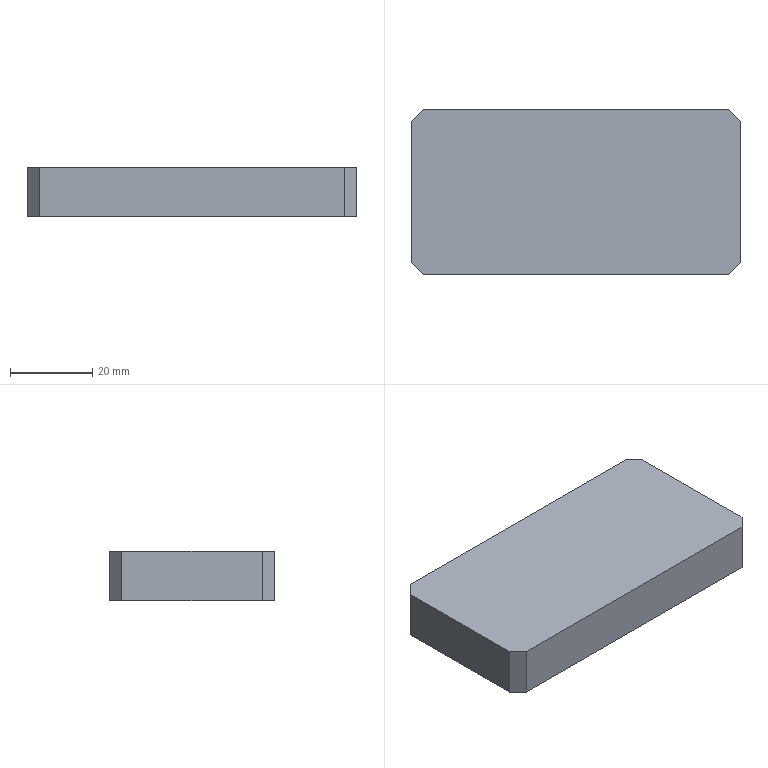Part | STEP file | 001-001-Small mounting plate | 1 solid | 10 faces | box 80 x 40 x 12 mm | volume 38184 mm3 | plane 10
STEP:
#1=CARTESIAN_POINT('',(0.,0.,0.));
#2=DIRECTION('',(0.,0.,1.));
#3=DIRECTION('',(1.,0.,0.));
#4=AXIS2_PLACEMENT_3D('',#1,#2,#3);
#5=CARTESIAN_POINT('',(-773.,430.,12.));
#6=VERTEX_POINT('',#5);
#7=CARTESIAN_POINT('',(-847.,430.,12.));
#8=VERTEX_POINT('',#7);
#9=CARTESIAN_POINT('',(-770.,430.,12.));
#10=DIRECTION('',(-1.,0.,0.));
#11=VECTOR('',#10,1.);
#12=LINE('',#9,#11);
#13=CARTESIAN_POINT('',(-770.,430.,12.));
#14=DIRECTION('',(0.,-1.,0.));
#15=DIRECTION('',(0.,0.,-1.));
#16=AXIS2_PLACEMENT_3D('',#13,#14,#15);
#17=PLANE('',#16);
#18=CARTESIAN_POINT('',(0.,0.));
#19=DIRECTION('',(0.,-1.));
#20=VECTOR('',#19,1.);
#21=LINE('',#18,#20);
#22=(GEOMETRIC_REPRESENTATION_CONTEXT(2)PARAMETRIC_REPRESENTATION_CONTEXT()REPRESENTATION_CONTEXT('',''));
#23=DEFINITIONAL_REPRESENTATION('',(#21),#22);
#24=PCURVE('',#17,#23);
#25=CARTESIAN_POINT('',(0.,0.,12.));
#26=DIRECTION('',(0.,0.,-1.));
#27=DIRECTION('',(-1.,0.,0.));
#28=AXIS2_PLACEMENT_3D('',#25,#26,#27);
#29=PLANE('',#28);
#30=CARTESIAN_POINT('',(770.,430.));
#31=DIRECTION('',(1.,0.));
#32=VECTOR('',#31,1.);
#33=LINE('',#30,#32);
#34=(GEOMETRIC_REPRESENTATION_CONTEXT(2)PARAMETRIC_REPRESENTATION_CONTEXT()REPRESENTATION_CONTEXT('',''));
#35=DEFINITIONAL_REPRESENTATION('',(#33),#34);
#36=PCURVE('',#29,#35);
#37=SURFACE_CURVE('',#12,(#24,#36),.PCURVE_S1.);
#38=EDGE_CURVE('',#6,#8,#37,.T.);
#39=ORIENTED_EDGE('',*,*,#38,.T.);
#40=CARTESIAN_POINT('',(-847.,430.,0.));
#41=VERTEX_POINT('',#40);
#42=CARTESIAN_POINT('',(-847.,430.,12.));
#43=DIRECTION('',(0.,0.,-1.));
#44=VECTOR('',#43,1.);
#45=LINE('',#42,#44);
#46=CARTESIAN_POINT('',(0.,-77.));
#47=DIRECTION('',(1.,0.));
#48=VECTOR('',#47,1.);
#49=LINE('',#46,#48);
#50=(GEOMETRIC_REPRESENTATION_CONTEXT(2)PARAMETRIC_REPRESENTATION_CONTEXT()REPRESENTATION_CONTEXT('',''));
#51=DEFINITIONAL_REPRESENTATION('',(#49),#50);
#52=PCURVE('',#17,#51);
#53=CARTESIAN_POINT('',(-847.,430.,12.));
#54=DIRECTION('',(0.7071,0.7071,0.));
#55=DIRECTION('',(0.,0.,-1.));
#56=AXIS2_PLACEMENT_3D('',#53,#54,#55);
#57=PLANE('',#56);
#58=CARTESIAN_POINT('',(0.,0.));
#59=DIRECTION('',(1.,0.));
#60=VECTOR('',#59,1.);
#61=LINE('',#58,#60);
#62=(GEOMETRIC_REPRESENTATION_CONTEXT(2)PARAMETRIC_REPRESENTATION_CONTEXT()REPRESENTATION_CONTEXT('',''));
#63=DEFINITIONAL_REPRESENTATION('',(#61),#62);
#64=PCURVE('',#57,#63);
#65=SURFACE_CURVE('',#45,(#52,#64),.PCURVE_S1.);
#66=EDGE_CURVE('',#8,#41,#65,.T.);
#67=ORIENTED_EDGE('',*,*,#66,.T.);
#68=CARTESIAN_POINT('',(-773.,430.,0.));
#69=VERTEX_POINT('',#68);
#70=CARTESIAN_POINT('',(-770.,430.,0.));
#71=DIRECTION('',(-1.,0.,0.));
#72=VECTOR('',#71,1.);
#73=LINE('',#70,#72);
#74=CARTESIAN_POINT('',(12.,0.));
#75=DIRECTION('',(0.,-1.));
#76=VECTOR('',#75,1.);
#77=LINE('',#74,#76);
#78=(GEOMETRIC_REPRESENTATION_CONTEXT(2)PARAMETRIC_REPRESENTATION_CONTEXT()REPRESENTATION_CONTEXT('',''));
#79=DEFINITIONAL_REPRESENTATION('',(#77),#78);
#80=PCURVE('',#17,#79);
#81=CARTESIAN_POINT('',(0.,0.,0.));
#82=DIRECTION('',(0.,0.,-1.));
#83=DIRECTION('',(-1.,0.,0.));
#84=AXIS2_PLACEMENT_3D('',#81,#82,#83);
#85=PLANE('',#84);
#86=CARTESIAN_POINT('',(770.,430.));
#87=DIRECTION('',(1.,0.));
#88=VECTOR('',#87,1.);
#89=LINE('',#86,#88);
#90=(GEOMETRIC_REPRESENTATION_CONTEXT(2)PARAMETRIC_REPRESENTATION_CONTEXT()REPRESENTATION_CONTEXT('',''));
#91=DEFINITIONAL_REPRESENTATION('',(#89),#90);
#92=PCURVE('',#85,#91);
#93=SURFACE_CURVE('',#73,(#80,#92),.PCURVE_S1.);
#94=EDGE_CURVE('',#69,#41,#93,.T.);
#95=ORIENTED_EDGE('',*,*,#94,.F.);
#96=CARTESIAN_POINT('',(-773.,430.,12.));
#97=DIRECTION('',(0.,0.,1.));
#98=VECTOR('',#97,1.);
#99=LINE('',#96,#98);
#100=CARTESIAN_POINT('',(0.,-3.));
#101=DIRECTION('',(-1.,0.));
#102=VECTOR('',#101,1.);
#103=LINE('',#100,#102);
#104=(GEOMETRIC_REPRESENTATION_CONTEXT(2)PARAMETRIC_REPRESENTATION_CONTEXT()REPRESENTATION_CONTEXT('',''));
#105=DEFINITIONAL_REPRESENTATION('',(#103),#104);
#106=PCURVE('',#17,#105);
#107=CARTESIAN_POINT('',(-770.,433.,12.));
#108=DIRECTION('',(0.7071,-0.7071,0.));
#109=DIRECTION('',(0.,0.,1.));
#110=AXIS2_PLACEMENT_3D('',#107,#108,#109);
#111=PLANE('',#110);
#112=CARTESIAN_POINT('',(0.,4.243));
#113=DIRECTION('',(1.,0.));
#114=VECTOR('',#113,1.);
#115=LINE('',#112,#114);
#116=(GEOMETRIC_REPRESENTATION_CONTEXT(2)PARAMETRIC_REPRESENTATION_CONTEXT()REPRESENTATION_CONTEXT('',''));
#117=DEFINITIONAL_REPRESENTATION('',(#115),#116);
#118=PCURVE('',#111,#117);
#119=SURFACE_CURVE('',#99,(#106,#118),.PCURVE_S1.);
#120=EDGE_CURVE('',#69,#6,#119,.T.);
#121=ORIENTED_EDGE('',*,*,#120,.T.);
#122=EDGE_LOOP('',(#39,#67,#95,#121));
#123=FACE_BOUND('',#122,.T.);
#124=ADVANCED_FACE('',(#123),#17,.T.);
#125=CARTESIAN_POINT('',(-770.,433.,12.));
#126=VERTEX_POINT('',#125);
#127=CARTESIAN_POINT('',(-770.,467.,12.));
#128=VERTEX_POINT('',#127);
#129=CARTESIAN_POINT('',(-770.,430.,12.));
#130=DIRECTION('',(0.,1.,0.));
#131=VECTOR('',#130,1.);
#132=LINE('',#129,#131);
#133=CARTESIAN_POINT('',(-770.,430.,12.));
#134=DIRECTION('',(-1.,0.,0.));
#135=DIRECTION('',(0.,0.,1.));
#136=AXIS2_PLACEMENT_3D('',#133,#134,#135);
#137=PLANE('',#136);
#138=CARTESIAN_POINT('',(0.,0.));
#139=DIRECTION('',(0.,1.));
#140=VECTOR('',#139,1.);
#141=LINE('',#138,#140);
#142=(GEOMETRIC_REPRESENTATION_CONTEXT(2)PARAMETRIC_REPRESENTATION_CONTEXT()REPRESENTATION_CONTEXT('',''));
#143=DEFINITIONAL_REPRESENTATION('',(#141),#142);
#144=PCURVE('',#137,#143);
#145=CARTESIAN_POINT('',(770.,430.));
#146=DIRECTION('',(0.,1.));
#147=VECTOR('',#146,1.);
#148=LINE('',#145,#147);
#149=(GEOMETRIC_REPRESENTATION_CONTEXT(2)PARAMETRIC_REPRESENTATION_CONTEXT()REPRESENTATION_CONTEXT('',''));
#150=DEFINITIONAL_REPRESENTATION('',(#148),#149);
#151=PCURVE('',#29,#150);
#152=SURFACE_CURVE('',#132,(#144,#151),.PCURVE_S1.);
#153=EDGE_CURVE('',#126,#128,#152,.T.);
#154=ORIENTED_EDGE('',*,*,#153,.F.);
#155=CARTESIAN_POINT('',(-770.,433.,0.));
#156=VERTEX_POINT('',#155);
#157=CARTESIAN_POINT('',(-770.,433.,0.));
#158=DIRECTION('',(0.,0.,-1.));
#159=VECTOR('',#158,1.);
#160=LINE('',#157,#159);
#161=CARTESIAN_POINT('',(-12.,3.));
#162=DIRECTION('',(-1.,0.));
#163=VECTOR('',#162,1.);
#164=LINE('',#161,#163);
#165=(GEOMETRIC_REPRESENTATION_CONTEXT(2)PARAMETRIC_REPRESENTATION_CONTEXT()REPRESENTATION_CONTEXT('',''));
#166=DEFINITIONAL_REPRESENTATION('',(#164),#165);
#167=PCURVE('',#137,#166);
#168=CARTESIAN_POINT('',(-12.,0.));
#169=DIRECTION('',(-1.,0.));
#170=VECTOR('',#169,1.);
#171=LINE('',#168,#170);
#172=(GEOMETRIC_REPRESENTATION_CONTEXT(2)PARAMETRIC_REPRESENTATION_CONTEXT()REPRESENTATION_CONTEXT('',''));
#173=DEFINITIONAL_REPRESENTATION('',(#171),#172);
#174=PCURVE('',#111,#173);
#175=SURFACE_CURVE('',#160,(#167,#174),.PCURVE_S1.);
#176=EDGE_CURVE('',#126,#156,#175,.T.);
#177=ORIENTED_EDGE('',*,*,#176,.T.);
#178=CARTESIAN_POINT('',(-770.,467.,0.));
#179=VERTEX_POINT('',#178);
#180=CARTESIAN_POINT('',(-770.,430.,0.));
#181=DIRECTION('',(0.,1.,0.));
#182=VECTOR('',#181,1.);
#183=LINE('',#180,#182);
#184=CARTESIAN_POINT('',(-12.,0.));
#185=DIRECTION('',(0.,1.));
#186=VECTOR('',#185,1.);
#187=LINE('',#184,#186);
#188=(GEOMETRIC_REPRESENTATION_CONTEXT(2)PARAMETRIC_REPRESENTATION_CONTEXT()REPRESENTATION_CONTEXT('',''));
#189=DEFINITIONAL_REPRESENTATION('',(#187),#188);
#190=PCURVE('',#137,#189);
#191=CARTESIAN_POINT('',(770.,430.));
#192=DIRECTION('',(0.,1.));
#193=VECTOR('',#192,1.);
#194=LINE('',#191,#193);
#195=(GEOMETRIC_REPRESENTATION_CONTEXT(2)PARAMETRIC_REPRESENTATION_CONTEXT()REPRESENTATION_CONTEXT('',''));
#196=DEFINITIONAL_REPRESENTATION('',(#194),#195);
#197=PCURVE('',#85,#196);
#198=SURFACE_CURVE('',#183,(#190,#197),.PCURVE_S1.);
#199=EDGE_CURVE('',#156,#179,#198,.T.);
#200=ORIENTED_EDGE('',*,*,#199,.T.);
#201=CARTESIAN_POINT('',(-770.,467.,12.));
#202=DIRECTION('',(0.,0.,1.));
#203=VECTOR('',#202,1.);
#204=LINE('',#201,#203);
#205=CARTESIAN_POINT('',(0.,37.));
#206=DIRECTION('',(1.,0.));
#207=VECTOR('',#206,1.);
#208=LINE('',#205,#207);
#209=(GEOMETRIC_REPRESENTATION_CONTEXT(2)PARAMETRIC_REPRESENTATION_CONTEXT()REPRESENTATION_CONTEXT('',''));
#210=DEFINITIONAL_REPRESENTATION('',(#208),#209);
#211=PCURVE('',#137,#210);
#212=CARTESIAN_POINT('',(-773.,470.,12.));
#213=DIRECTION('',(-0.7071,-0.7071,0.));
#214=DIRECTION('',(0.,0.,-1.));
#215=AXIS2_PLACEMENT_3D('',#212,#213,#214);
#216=PLANE('',#215);
#217=CARTESIAN_POINT('',(0.,4.243));
#218=DIRECTION('',(-1.,0.));
#219=VECTOR('',#218,1.);
#220=LINE('',#217,#219);
#221=(GEOMETRIC_REPRESENTATION_CONTEXT(2)PARAMETRIC_REPRESENTATION_CONTEXT()REPRESENTATION_CONTEXT('',''));
#222=DEFINITIONAL_REPRESENTATION('',(#220),#221);
#223=PCURVE('',#216,#222);
#224=SURFACE_CURVE('',#204,(#211,#223),.PCURVE_S1.);
#225=EDGE_CURVE('',#179,#128,#224,.T.);
#226=ORIENTED_EDGE('',*,*,#225,.T.);
#227=EDGE_LOOP('',(#154,#177,#200,#226));
#228=FACE_BOUND('',#227,.T.);
#229=ADVANCED_FACE('',(#228),#137,.F.);
#230=CARTESIAN_POINT('',(-773.,470.,0.));
#231=VERTEX_POINT('',#230);
#232=CARTESIAN_POINT('',(-847.,470.,0.));
#233=VERTEX_POINT('',#232);
#234=CARTESIAN_POINT('',(-770.,470.,0.));
#235=DIRECTION('',(-1.,0.,0.));
#236=VECTOR('',#235,1.);
#237=LINE('',#234,#236);
#238=CARTESIAN_POINT('',(-770.,470.,12.));
#239=DIRECTION('',(0.,-1.,0.));
#240=DIRECTION('',(0.,0.,-1.));
#241=AXIS2_PLACEMENT_3D('',#238,#239,#240);
#242=PLANE('',#241);
#243=CARTESIAN_POINT('',(12.,0.));
#244=DIRECTION('',(0.,-1.));
#245=VECTOR('',#244,1.);
#246=LINE('',#243,#245);
#247=(GEOMETRIC_REPRESENTATION_CONTEXT(2)PARAMETRIC_REPRESENTATION_CONTEXT()REPRESENTATION_CONTEXT('',''));
#248=DEFINITIONAL_REPRESENTATION('',(#246),#247);
#249=PCURVE('',#242,#248);
#250=CARTESIAN_POINT('',(770.,470.));
#251=DIRECTION('',(1.,0.));
#252=VECTOR('',#251,1.);
#253=LINE('',#250,#252);
#254=(GEOMETRIC_REPRESENTATION_CONTEXT(2)PARAMETRIC_REPRESENTATION_CONTEXT()REPRESENTATION_CONTEXT('',''));
#255=DEFINITIONAL_REPRESENTATION('',(#253),#254);
#256=PCURVE('',#85,#255);
#257=SURFACE_CURVE('',#237,(#249,#256),.PCURVE_S1.);
#258=EDGE_CURVE('',#231,#233,#257,.T.);
#259=ORIENTED_EDGE('',*,*,#258,.T.);
#260=CARTESIAN_POINT('',(-847.,470.,12.));
#261=VERTEX_POINT('',#260);
#262=CARTESIAN_POINT('',(-847.,470.,12.));
#263=DIRECTION('',(0.,0.,1.));
#264=VECTOR('',#263,1.);
#265=LINE('',#262,#264);
#266=CARTESIAN_POINT('',(0.,-77.));
#267=DIRECTION('',(-1.,0.));
#268=VECTOR('',#267,1.);
#269=LINE('',#266,#268);
#270=(GEOMETRIC_REPRESENTATION_CONTEXT(2)PARAMETRIC_REPRESENTATION_CONTEXT()REPRESENTATION_CONTEXT('',''));
#271=DEFINITIONAL_REPRESENTATION('',(#269),#270);
#272=PCURVE('',#242,#271);
#273=CARTESIAN_POINT('',(-850.,467.,12.));
#274=DIRECTION('',(-0.7071,0.7071,0.));
#275=DIRECTION('',(0.,0.,1.));
#276=AXIS2_PLACEMENT_3D('',#273,#274,#275);
#277=PLANE('',#276);
#278=CARTESIAN_POINT('',(0.,4.243));
#279=DIRECTION('',(1.,0.));
#280=VECTOR('',#279,1.);
#281=LINE('',#278,#280);
#282=(GEOMETRIC_REPRESENTATION_CONTEXT(2)PARAMETRIC_REPRESENTATION_CONTEXT()REPRESENTATION_CONTEXT('',''));
#283=DEFINITIONAL_REPRESENTATION('',(#281),#282);
#284=PCURVE('',#277,#283);
#285=SURFACE_CURVE('',#265,(#272,#284),.PCURVE_S1.);
#286=EDGE_CURVE('',#233,#261,#285,.T.);
#287=ORIENTED_EDGE('',*,*,#286,.T.);
#288=CARTESIAN_POINT('',(-773.,470.,12.));
#289=VERTEX_POINT('',#288);
#290=CARTESIAN_POINT('',(-770.,470.,12.));
#291=DIRECTION('',(-1.,0.,0.));
#292=VECTOR('',#291,1.);
#293=LINE('',#290,#292);
#294=CARTESIAN_POINT('',(0.,0.));
#295=DIRECTION('',(0.,-1.));
#296=VECTOR('',#295,1.);
#297=LINE('',#294,#296);
#298=(GEOMETRIC_REPRESENTATION_CONTEXT(2)PARAMETRIC_REPRESENTATION_CONTEXT()REPRESENTATION_CONTEXT('',''));
#299=DEFINITIONAL_REPRESENTATION('',(#297),#298);
#300=PCURVE('',#242,#299);
#301=CARTESIAN_POINT('',(770.,470.));
#302=DIRECTION('',(1.,0.));
#303=VECTOR('',#302,1.);
#304=LINE('',#301,#303);
#305=(GEOMETRIC_REPRESENTATION_CONTEXT(2)PARAMETRIC_REPRESENTATION_CONTEXT()REPRESENTATION_CONTEXT('',''));
#306=DEFINITIONAL_REPRESENTATION('',(#304),#305);
#307=PCURVE('',#29,#306);
#308=SURFACE_CURVE('',#293,(#300,#307),.PCURVE_S1.);
#309=EDGE_CURVE('',#289,#261,#308,.T.);
#310=ORIENTED_EDGE('',*,*,#309,.F.);
#311=CARTESIAN_POINT('',(-773.,470.,12.));
#312=DIRECTION('',(0.,0.,-1.));
#313=VECTOR('',#312,1.);
#314=LINE('',#311,#313);
#315=CARTESIAN_POINT('',(0.,-3.));
#316=DIRECTION('',(1.,0.));
#317=VECTOR('',#316,1.);
#318=LINE('',#315,#317);
#319=(GEOMETRIC_REPRESENTATION_CONTEXT(2)PARAMETRIC_REPRESENTATION_CONTEXT()REPRESENTATION_CONTEXT('',''));
#320=DEFINITIONAL_REPRESENTATION('',(#318),#319);
#321=PCURVE('',#242,#320);
#322=CARTESIAN_POINT('',(0.,0.));
#323=DIRECTION('',(1.,0.));
#324=VECTOR('',#323,1.);
#325=LINE('',#322,#324);
#326=(GEOMETRIC_REPRESENTATION_CONTEXT(2)PARAMETRIC_REPRESENTATION_CONTEXT()REPRESENTATION_CONTEXT('',''));
#327=DEFINITIONAL_REPRESENTATION('',(#325),#326);
#328=PCURVE('',#216,#327);
#329=SURFACE_CURVE('',#314,(#321,#328),.PCURVE_S1.);
#330=EDGE_CURVE('',#289,#231,#329,.T.);
#331=ORIENTED_EDGE('',*,*,#330,.T.);
#332=EDGE_LOOP('',(#259,#287,#310,#331));
#333=FACE_BOUND('',#332,.T.);
#334=ADVANCED_FACE('',(#333),#242,.F.);
#335=CARTESIAN_POINT('',(-850.,433.,0.));
#336=VERTEX_POINT('',#335);
#337=CARTESIAN_POINT('',(-850.,467.,0.));
#338=VERTEX_POINT('',#337);
#339=CARTESIAN_POINT('',(-850.,430.,0.));
#340=DIRECTION('',(0.,1.,0.));
#341=VECTOR('',#340,1.);
#342=LINE('',#339,#341);
#343=CARTESIAN_POINT('',(-850.,430.,12.));
#344=DIRECTION('',(-1.,0.,0.));
#345=DIRECTION('',(0.,0.,1.));
#346=AXIS2_PLACEMENT_3D('',#343,#344,#345);
#347=PLANE('',#346);
#348=CARTESIAN_POINT('',(-12.,0.));
#349=DIRECTION('',(0.,1.));
#350=VECTOR('',#349,1.);
#351=LINE('',#348,#350);
#352=(GEOMETRIC_REPRESENTATION_CONTEXT(2)PARAMETRIC_REPRESENTATION_CONTEXT()REPRESENTATION_CONTEXT('',''));
#353=DEFINITIONAL_REPRESENTATION('',(#351),#352);
#354=PCURVE('',#347,#353);
#355=CARTESIAN_POINT('',(850.,430.));
#356=DIRECTION('',(0.,1.));
#357=VECTOR('',#356,1.);
#358=LINE('',#355,#357);
#359=(GEOMETRIC_REPRESENTATION_CONTEXT(2)PARAMETRIC_REPRESENTATION_CONTEXT()REPRESENTATION_CONTEXT('',''));
#360=DEFINITIONAL_REPRESENTATION('',(#358),#359);
#361=PCURVE('',#85,#360);
#362=SURFACE_CURVE('',#342,(#354,#361),.PCURVE_S1.);
#363=EDGE_CURVE('',#336,#338,#362,.T.);
#364=ORIENTED_EDGE('',*,*,#363,.F.);
#365=CARTESIAN_POINT('',(-850.,433.,12.));
#366=VERTEX_POINT('',#365);
#367=CARTESIAN_POINT('',(-850.,433.,12.));
#368=DIRECTION('',(0.,0.,1.));
#369=VECTOR('',#368,1.);
#370=LINE('',#367,#369);
#371=CARTESIAN_POINT('',(0.,3.));
#372=DIRECTION('',(1.,0.));
#373=VECTOR('',#372,1.);
#374=LINE('',#371,#373);
#375=(GEOMETRIC_REPRESENTATION_CONTEXT(2)PARAMETRIC_REPRESENTATION_CONTEXT()REPRESENTATION_CONTEXT('',''));
#376=DEFINITIONAL_REPRESENTATION('',(#374),#375);
#377=PCURVE('',#347,#376);
#378=CARTESIAN_POINT('',(0.,4.243));
#379=DIRECTION('',(-1.,0.));
#380=VECTOR('',#379,1.);
#381=LINE('',#378,#380);
#382=(GEOMETRIC_REPRESENTATION_CONTEXT(2)PARAMETRIC_REPRESENTATION_CONTEXT()REPRESENTATION_CONTEXT('',''));
#383=DEFINITIONAL_REPRESENTATION('',(#381),#382);
#384=PCURVE('',#57,#383);
#385=SURFACE_CURVE('',#370,(#377,#384),.PCURVE_S1.);
#386=EDGE_CURVE('',#336,#366,#385,.T.);
#387=ORIENTED_EDGE('',*,*,#386,.T.);
#388=CARTESIAN_POINT('',(-850.,467.,12.));
#389=VERTEX_POINT('',#388);
#390=CARTESIAN_POINT('',(-850.,430.,12.));
#391=DIRECTION('',(0.,1.,0.));
#392=VECTOR('',#391,1.);
#393=LINE('',#390,#392);
#394=CARTESIAN_POINT('',(0.,0.));
#395=DIRECTION('',(0.,1.));
#396=VECTOR('',#395,1.);
#397=LINE('',#394,#396);
#398=(GEOMETRIC_REPRESENTATION_CONTEXT(2)PARAMETRIC_REPRESENTATION_CONTEXT()REPRESENTATION_CONTEXT('',''));
#399=DEFINITIONAL_REPRESENTATION('',(#397),#398);
#400=PCURVE('',#347,#399);
#401=CARTESIAN_POINT('',(850.,430.));
#402=DIRECTION('',(0.,1.));
#403=VECTOR('',#402,1.);
#404=LINE('',#401,#403);
#405=(GEOMETRIC_REPRESENTATION_CONTEXT(2)PARAMETRIC_REPRESENTATION_CONTEXT()REPRESENTATION_CONTEXT('',''));
#406=DEFINITIONAL_REPRESENTATION('',(#404),#405);
#407=PCURVE('',#29,#406);
#408=SURFACE_CURVE('',#393,(#400,#407),.PCURVE_S1.);
#409=EDGE_CURVE('',#366,#389,#408,.T.);
#410=ORIENTED_EDGE('',*,*,#409,.T.);
#411=CARTESIAN_POINT('',(-850.,467.,0.));
#412=DIRECTION('',(0.,0.,-1.));
#413=VECTOR('',#412,1.);
#414=LINE('',#411,#413);
#415=CARTESIAN_POINT('',(-12.,37.));
#416=DIRECTION('',(-1.,0.));
#417=VECTOR('',#416,1.);
#418=LINE('',#415,#417);
#419=(GEOMETRIC_REPRESENTATION_CONTEXT(2)PARAMETRIC_REPRESENTATION_CONTEXT()REPRESENTATION_CONTEXT('',''));
#420=DEFINITIONAL_REPRESENTATION('',(#418),#419);
#421=PCURVE('',#347,#420);
#422=CARTESIAN_POINT('',(-12.,0.));
#423=DIRECTION('',(-1.,0.));
#424=VECTOR('',#423,1.);
#425=LINE('',#422,#424);
#426=(GEOMETRIC_REPRESENTATION_CONTEXT(2)PARAMETRIC_REPRESENTATION_CONTEXT()REPRESENTATION_CONTEXT('',''));
#427=DEFINITIONAL_REPRESENTATION('',(#425),#426);
#428=PCURVE('',#277,#427);
#429=SURFACE_CURVE('',#414,(#421,#428),.PCURVE_S1.);
#430=EDGE_CURVE('',#389,#338,#429,.T.);
#431=ORIENTED_EDGE('',*,*,#430,.T.);
#432=EDGE_LOOP('',(#364,#387,#410,#431));
#433=FACE_BOUND('',#432,.T.);
#434=ADVANCED_FACE('',(#433),#347,.T.);
#435=ORIENTED_EDGE('',*,*,#409,.F.);
#436=CARTESIAN_POINT('',(-847.,430.,12.));
#437=DIRECTION('',(0.7071,-0.7071,0.));
#438=VECTOR('',#437,1.);
#439=LINE('',#436,#438);
#440=CARTESIAN_POINT('',(847.,430.));
#441=DIRECTION('',(-0.7071,-0.7071));
#442=VECTOR('',#441,1.);
#443=LINE('',#440,#442);
#444=(GEOMETRIC_REPRESENTATION_CONTEXT(2)PARAMETRIC_REPRESENTATION_CONTEXT()REPRESENTATION_CONTEXT('',''));
#445=DEFINITIONAL_REPRESENTATION('',(#443),#444);
#446=PCURVE('',#29,#445);
#447=CARTESIAN_POINT('',(0.,0.));
#448=DIRECTION('',(0.,-1.));
#449=VECTOR('',#448,1.);
#450=LINE('',#447,#449);
#451=(GEOMETRIC_REPRESENTATION_CONTEXT(2)PARAMETRIC_REPRESENTATION_CONTEXT()REPRESENTATION_CONTEXT('',''));
#452=DEFINITIONAL_REPRESENTATION('',(#450),#451);
#453=PCURVE('',#57,#452);
#454=SURFACE_CURVE('',#439,(#446,#453),.PCURVE_S1.);
#455=EDGE_CURVE('',#366,#8,#454,.T.);
#456=ORIENTED_EDGE('',*,*,#455,.T.);
#457=ORIENTED_EDGE('',*,*,#38,.F.);
#458=CARTESIAN_POINT('',(-770.,433.,12.));
#459=DIRECTION('',(0.7071,0.7071,0.));
#460=VECTOR('',#459,1.);
#461=LINE('',#458,#460);
#462=CARTESIAN_POINT('',(770.,433.));
#463=DIRECTION('',(-0.7071,0.7071));
#464=VECTOR('',#463,1.);
#465=LINE('',#462,#464);
#466=(GEOMETRIC_REPRESENTATION_CONTEXT(2)PARAMETRIC_REPRESENTATION_CONTEXT()REPRESENTATION_CONTEXT('',''));
#467=DEFINITIONAL_REPRESENTATION('',(#465),#466);
#468=PCURVE('',#29,#467);
#469=CARTESIAN_POINT('',(0.,0.));
#470=DIRECTION('',(0.,-1.));
#471=VECTOR('',#470,1.);
#472=LINE('',#469,#471);
#473=(GEOMETRIC_REPRESENTATION_CONTEXT(2)PARAMETRIC_REPRESENTATION_CONTEXT()REPRESENTATION_CONTEXT('',''));
#474=DEFINITIONAL_REPRESENTATION('',(#472),#473);
#475=PCURVE('',#111,#474);
#476=SURFACE_CURVE('',#461,(#468,#475),.PCURVE_S1.);
#477=EDGE_CURVE('',#6,#126,#476,.T.);
#478=ORIENTED_EDGE('',*,*,#477,.T.);
#479=ORIENTED_EDGE('',*,*,#153,.T.);
#480=CARTESIAN_POINT('',(-773.,470.,12.));
#481=DIRECTION('',(-0.7071,0.7071,0.));
#482=VECTOR('',#481,1.);
#483=LINE('',#480,#482);
#484=CARTESIAN_POINT('',(773.,470.));
#485=DIRECTION('',(0.7071,0.7071));
#486=VECTOR('',#485,1.);
#487=LINE('',#484,#486);
#488=(GEOMETRIC_REPRESENTATION_CONTEXT(2)PARAMETRIC_REPRESENTATION_CONTEXT()REPRESENTATION_CONTEXT('',''));
#489=DEFINITIONAL_REPRESENTATION('',(#487),#488);
#490=PCURVE('',#29,#489);
#491=CARTESIAN_POINT('',(0.,0.));
#492=DIRECTION('',(0.,-1.));
#493=VECTOR('',#492,1.);
#494=LINE('',#491,#493);
#495=(GEOMETRIC_REPRESENTATION_CONTEXT(2)PARAMETRIC_REPRESENTATION_CONTEXT()REPRESENTATION_CONTEXT('',''));
#496=DEFINITIONAL_REPRESENTATION('',(#494),#495);
#497=PCURVE('',#216,#496);
#498=SURFACE_CURVE('',#483,(#490,#497),.PCURVE_S1.);
#499=EDGE_CURVE('',#128,#289,#498,.T.);
#500=ORIENTED_EDGE('',*,*,#499,.T.);
#501=ORIENTED_EDGE('',*,*,#309,.T.);
#502=CARTESIAN_POINT('',(-850.,467.,12.));
#503=DIRECTION('',(-0.7071,-0.7071,0.));
#504=VECTOR('',#503,1.);
#505=LINE('',#502,#504);
#506=CARTESIAN_POINT('',(850.,467.));
#507=DIRECTION('',(0.7071,-0.7071));
#508=VECTOR('',#507,1.);
#509=LINE('',#506,#508);
#510=(GEOMETRIC_REPRESENTATION_CONTEXT(2)PARAMETRIC_REPRESENTATION_CONTEXT()REPRESENTATION_CONTEXT('',''));
#511=DEFINITIONAL_REPRESENTATION('',(#509),#510);
#512=PCURVE('',#29,#511);
#513=CARTESIAN_POINT('',(0.,0.));
#514=DIRECTION('',(0.,-1.));
#515=VECTOR('',#514,1.);
#516=LINE('',#513,#515);
#517=(GEOMETRIC_REPRESENTATION_CONTEXT(2)PARAMETRIC_REPRESENTATION_CONTEXT()REPRESENTATION_CONTEXT('',''));
#518=DEFINITIONAL_REPRESENTATION('',(#516),#517);
#519=PCURVE('',#277,#518);
#520=SURFACE_CURVE('',#505,(#512,#519),.PCURVE_S1.);
#521=EDGE_CURVE('',#261,#389,#520,.T.);
#522=ORIENTED_EDGE('',*,*,#521,.T.);
#523=EDGE_LOOP('',(#435,#456,#457,#478,#479,#500,#501,#522));
#524=FACE_BOUND('',#523,.T.);
#525=ADVANCED_FACE('',(#524),#29,.F.);
#526=ORIENTED_EDGE('',*,*,#94,.T.);
#527=CARTESIAN_POINT('',(-208.5,-208.5,0.));
#528=DIRECTION('',(-0.7071,0.7071,0.));
#529=VECTOR('',#528,1.);
#530=LINE('',#527,#529);
#531=CARTESIAN_POINT('',(208.5,-208.5));
#532=DIRECTION('',(0.7071,0.7071));
#533=VECTOR('',#532,1.);
#534=LINE('',#531,#533);
#535=(GEOMETRIC_REPRESENTATION_CONTEXT(2)PARAMETRIC_REPRESENTATION_CONTEXT()REPRESENTATION_CONTEXT('',''));
#536=DEFINITIONAL_REPRESENTATION('',(#534),#535);
#537=PCURVE('',#85,#536);
#538=CARTESIAN_POINT('',(12.,-902.975));
#539=DIRECTION('',(0.,1.));
#540=VECTOR('',#539,1.);
#541=LINE('',#538,#540);
#542=(GEOMETRIC_REPRESENTATION_CONTEXT(2)PARAMETRIC_REPRESENTATION_CONTEXT()REPRESENTATION_CONTEXT('',''));
#543=DEFINITIONAL_REPRESENTATION('',(#541),#542);
#544=PCURVE('',#57,#543);
#545=SURFACE_CURVE('',#530,(#537,#544),.PCURVE_S1.);
#546=EDGE_CURVE('',#41,#336,#545,.T.);
#547=ORIENTED_EDGE('',*,*,#546,.T.);
#548=ORIENTED_EDGE('',*,*,#363,.T.);
#549=CARTESIAN_POINT('',(-658.5,658.5,0.));
#550=DIRECTION('',(0.7071,0.7071,0.));
#551=VECTOR('',#550,1.);
#552=LINE('',#549,#551);
#553=CARTESIAN_POINT('',(658.5,658.5));
#554=DIRECTION('',(-0.7071,0.7071));
#555=VECTOR('',#554,1.);
#556=LINE('',#553,#555);
#557=(GEOMETRIC_REPRESENTATION_CONTEXT(2)PARAMETRIC_REPRESENTATION_CONTEXT()REPRESENTATION_CONTEXT('',''));
#558=DEFINITIONAL_REPRESENTATION('',(#556),#557);
#559=PCURVE('',#85,#558);
#560=CARTESIAN_POINT('',(-12.,270.822));
#561=DIRECTION('',(0.,1.));
#562=VECTOR('',#561,1.);
#563=LINE('',#560,#562);
#564=(GEOMETRIC_REPRESENTATION_CONTEXT(2)PARAMETRIC_REPRESENTATION_CONTEXT()REPRESENTATION_CONTEXT('',''));
#565=DEFINITIONAL_REPRESENTATION('',(#563),#564);
#566=PCURVE('',#277,#565);
#567=SURFACE_CURVE('',#552,(#559,#566),.PCURVE_S1.);
#568=EDGE_CURVE('',#338,#233,#567,.T.);
#569=ORIENTED_EDGE('',*,*,#568,.T.);
#570=ORIENTED_EDGE('',*,*,#258,.F.);
#571=CARTESIAN_POINT('',(-151.5,-151.5,0.));
#572=DIRECTION('',(0.7071,-0.7071,0.));
#573=VECTOR('',#572,1.);
#574=LINE('',#571,#573);
#575=CARTESIAN_POINT('',(151.5,-151.5));
#576=DIRECTION('',(-0.7071,-0.7071));
#577=VECTOR('',#576,1.);
#578=LINE('',#575,#577);
#579=(GEOMETRIC_REPRESENTATION_CONTEXT(2)PARAMETRIC_REPRESENTATION_CONTEXT()REPRESENTATION_CONTEXT('',''));
#580=DEFINITIONAL_REPRESENTATION('',(#578),#579);
#581=PCURVE('',#85,#580);
#582=CARTESIAN_POINT('',(12.,878.934));
#583=DIRECTION('',(0.,1.));
#584=VECTOR('',#583,1.);
#585=LINE('',#582,#584);
#586=(GEOMETRIC_REPRESENTATION_CONTEXT(2)PARAMETRIC_REPRESENTATION_CONTEXT()REPRESENTATION_CONTEXT('',''));
#587=DEFINITIONAL_REPRESENTATION('',(#585),#586);
#588=PCURVE('',#216,#587);
#589=SURFACE_CURVE('',#574,(#581,#588),.PCURVE_S1.);
#590=EDGE_CURVE('',#231,#179,#589,.T.);
#591=ORIENTED_EDGE('',*,*,#590,.T.);
#592=ORIENTED_EDGE('',*,*,#199,.F.);
#593=CARTESIAN_POINT('',(-601.5,601.5,0.));
#594=DIRECTION('',(-0.7071,-0.7071,0.));
#595=VECTOR('',#594,1.);
#596=LINE('',#593,#595);
#597=CARTESIAN_POINT('',(601.5,601.5));
#598=DIRECTION('',(0.7071,-0.7071));
#599=VECTOR('',#598,1.);
#600=LINE('',#597,#599);
#601=(GEOMETRIC_REPRESENTATION_CONTEXT(2)PARAMETRIC_REPRESENTATION_CONTEXT()REPRESENTATION_CONTEXT('',''));
#602=DEFINITIONAL_REPRESENTATION('',(#600),#601);
#603=PCURVE('',#85,#602);
#604=CARTESIAN_POINT('',(-12.,-238.295));
#605=DIRECTION('',(0.,1.));
#606=VECTOR('',#605,1.);
#607=LINE('',#604,#606);
#608=(GEOMETRIC_REPRESENTATION_CONTEXT(2)PARAMETRIC_REPRESENTATION_CONTEXT()REPRESENTATION_CONTEXT('',''));
#609=DEFINITIONAL_REPRESENTATION('',(#607),#608);
#610=PCURVE('',#111,#609);
#611=SURFACE_CURVE('',#596,(#603,#610),.PCURVE_S1.);
#612=EDGE_CURVE('',#156,#69,#611,.T.);
#613=ORIENTED_EDGE('',*,*,#612,.T.);
#614=EDGE_LOOP('',(#526,#547,#548,#569,#570,#591,#592,#613));
#615=FACE_BOUND('',#614,.T.);
#616=ADVANCED_FACE('',(#615),#85,.T.);
#617=ORIENTED_EDGE('',*,*,#455,.F.);
#618=ORIENTED_EDGE('',*,*,#386,.F.);
#619=ORIENTED_EDGE('',*,*,#546,.F.);
#620=ORIENTED_EDGE('',*,*,#66,.F.);
#621=EDGE_LOOP('',(#617,#618,#619,#620));
#622=FACE_BOUND('',#621,.T.);
#623=ADVANCED_FACE('',(#622),#57,.F.);
#624=ORIENTED_EDGE('',*,*,#521,.F.);
#625=ORIENTED_EDGE('',*,*,#286,.F.);
#626=ORIENTED_EDGE('',*,*,#568,.F.);
#627=ORIENTED_EDGE('',*,*,#430,.F.);
#628=EDGE_LOOP('',(#624,#625,#626,#627));
#629=FACE_BOUND('',#628,.T.);
#630=ADVANCED_FACE('',(#629),#277,.T.);
#631=ORIENTED_EDGE('',*,*,#477,.F.);
#632=ORIENTED_EDGE('',*,*,#120,.F.);
#633=ORIENTED_EDGE('',*,*,#612,.F.);
#634=ORIENTED_EDGE('',*,*,#176,.F.);
#635=EDGE_LOOP('',(#631,#632,#633,#634));
#636=FACE_BOUND('',#635,.T.);
#637=ADVANCED_FACE('',(#636),#111,.T.);
#638=ORIENTED_EDGE('',*,*,#499,.F.);
#639=ORIENTED_EDGE('',*,*,#225,.F.);
#640=ORIENTED_EDGE('',*,*,#590,.F.);
#641=ORIENTED_EDGE('',*,*,#330,.F.);
#642=EDGE_LOOP('',(#638,#639,#640,#641));
#643=FACE_BOUND('',#642,.T.);
#644=ADVANCED_FACE('',(#643),#216,.F.);
#645=CLOSED_SHELL('',(#124,#229,#334,#434,#525,#616,#623,#630,#637,#644));
#646=MANIFOLD_SOLID_BREP('',#645);
#647=(LENGTH_UNIT()NAMED_UNIT(*)SI_UNIT(.MILLI.,.METRE.));
#648=UNCERTAINTY_MEASURE_WITH_UNIT(LENGTH_MEASURE(0.0000001),#647,'','');
#649=(NAMED_UNIT(*)PLANE_ANGLE_UNIT()SI_UNIT($,.RADIAN.));
#650=(NAMED_UNIT(*)SI_UNIT($,.STERADIAN.)SOLID_ANGLE_UNIT());
#651=(GEOMETRIC_REPRESENTATION_CONTEXT(3)GLOBAL_UNCERTAINTY_ASSIGNED_CONTEXT((#648))GLOBAL_UNIT_ASSIGNED_CONTEXT((#647,#649,#650))REPRESENTATION_CONTEXT('',''));
#652=ADVANCED_BREP_SHAPE_REPRESENTATION('',(#4,#646),#651);